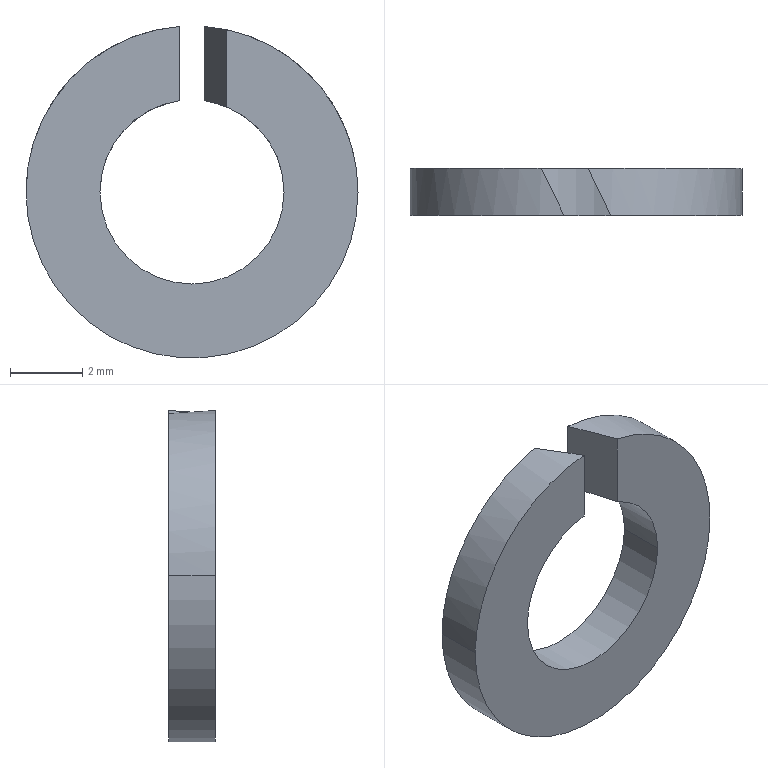Part | STEP file | ZZ24-M5 | 1 solid | 10 faces | box 9.2 x 1.3 x 9.188 mm | volume 56.371 mm3 | cylinder 6 | plane 4 | commonest cylinder face diameters 5.1 x3 9.2 x3
STEP:
#1=CARTESIAN_POINT('',(0.,0.,0.));
#2=DIRECTION('',(0.,0.,1.));
#3=DIRECTION('',(1.,0.,0.));
#4=AXIS2_PLACEMENT_3D('',#1,#2,#3);
#5=CARTESIAN_POINT('',(0.967,0.,2.36));
#6=VERTEX_POINT('',#5);
#7=CARTESIAN_POINT('',(0.333,1.3,2.528));
#8=VERTEX_POINT('',#7);
#9=CARTESIAN_POINT('',(0.967,0.,2.36));
#10=CARTESIAN_POINT('',(0.7635,0.4172,2.443));
#11=CARTESIAN_POINT('',(0.551,0.853,2.499));
#12=CARTESIAN_POINT('',(0.333,1.3,2.528));
#13=(BOUNDED_CURVE()B_SPLINE_CURVE(3,(#9,#10,#11,#12),.UNSPECIFIED.,.F.,.F.)B_SPLINE_CURVE_WITH_KNOTS((4,4),(1.182,1.44),.PIECEWISE_BEZIER_KNOTS.)CURVE()GEOMETRIC_REPRESENTATION_ITEM()RATIONAL_B_SPLINE_CURVE((1.,0.9945,0.9945,1.))REPRESENTATION_ITEM(''));
#14=CARTESIAN_POINT('',(0.,1.3,0.));
#15=DIRECTION('',(0.,-1.,0.));
#16=DIRECTION('',(-1.,0.,0.001512));
#17=AXIS2_PLACEMENT_3D('',#14,#15,#16);
#18=CYLINDRICAL_SURFACE('',#17,2.55);
#19=CARTESIAN_POINT('',(4.325,1.3));
#20=CARTESIAN_POINT('',(4.329,1.281));
#21=CARTESIAN_POINT('',(4.337,1.243));
#22=CARTESIAN_POINT('',(4.348,1.186));
#23=CARTESIAN_POINT('',(4.36,1.129));
#24=CARTESIAN_POINT('',(4.372,1.071));
#25=CARTESIAN_POINT('',(4.384,1.013));
#26=CARTESIAN_POINT('',(4.395,0.9553));
#27=CARTESIAN_POINT('',(4.407,0.8969));
#28=CARTESIAN_POINT('',(4.419,0.8383));
#29=CARTESIAN_POINT('',(4.43,0.7795));
#30=CARTESIAN_POINT('',(4.442,0.7204));
#31=CARTESIAN_POINT('',(4.454,0.6612));
#32=CARTESIAN_POINT('',(4.466,0.6018));
#33=CARTESIAN_POINT('',(4.477,0.5422));
#34=CARTESIAN_POINT('',(4.489,0.4824));
#35=CARTESIAN_POINT('',(4.501,0.4225));
#36=CARTESIAN_POINT('',(4.513,0.3624));
#37=CARTESIAN_POINT('',(4.524,0.3023));
#38=CARTESIAN_POINT('',(4.536,0.242));
#39=CARTESIAN_POINT('',(4.548,0.1816));
#40=CARTESIAN_POINT('',(4.56,0.1211));
#41=CARTESIAN_POINT('',(4.571,0.06061));
#42=CARTESIAN_POINT('',(4.579,0.02021));
#43=CARTESIAN_POINT('',(4.583,0.));
#44=B_SPLINE_CURVE_WITH_KNOTS('',3,(#19,#20,#21,#22,#23,#24,#25,#26,#27,#28,#29,#30,#31,#32,#33,#34,#35,#36,#37,#38,#39,#40,#41,#42,#43),.UNSPECIFIED.,.F.,.F.,(4,1,1,1,1,1,1,1,1,1,1,1,1,1,1,1,1,1,1,1,1,1,4),(1.182,1.194,1.205,1.217,1.229,1.24,1.252,1.264,1.276,1.287,1.299,1.311,1.323,1.334,1.346,1.358,1.369,1.381,1.393,1.405,1.416,1.428,1.44),.QUASI_UNIFORM_KNOTS.);
#45=(GEOMETRIC_REPRESENTATION_CONTEXT(2)PARAMETRIC_REPRESENTATION_CONTEXT()REPRESENTATION_CONTEXT('',''));
#46=DEFINITIONAL_REPRESENTATION('',(#44),#45);
#47=PCURVE('',#18,#46);
#48=CARTESIAN_POINT('',(0.967,0.,4.6));
#49=DIRECTION('',(-0.8988,-0.4384,0.));
#50=DIRECTION('',(0.4384,-0.8988,0.));
#51=AXIS2_PLACEMENT_3D('',#48,#49,#50);
#52=PLANE('',#51);
#53=CARTESIAN_POINT('',(0.,-2.24));
#54=CARTESIAN_POINT('',(-0.4642,-2.157));
#55=CARTESIAN_POINT('',(-0.949,-2.101));
#56=CARTESIAN_POINT('',(-1.446,-2.072));
#57=(BOUNDED_CURVE()B_SPLINE_CURVE(3,(#53,#54,#55,#56),.UNSPECIFIED.,.F.,.F.)B_SPLINE_CURVE_WITH_KNOTS((4,4),(1.182,1.44),.PIECEWISE_BEZIER_KNOTS.)CURVE()GEOMETRIC_REPRESENTATION_ITEM()RATIONAL_B_SPLINE_CURVE((1.,0.9945,0.9945,1.))REPRESENTATION_ITEM(''));
#58=(GEOMETRIC_REPRESENTATION_CONTEXT(2)PARAMETRIC_REPRESENTATION_CONTEXT()REPRESENTATION_CONTEXT('',''));
#59=DEFINITIONAL_REPRESENTATION('',(#57),#58);
#60=PCURVE('',#52,#59);
#61=SURFACE_CURVE('',#13,(#47,#60),.PCURVE_S1.);
#62=EDGE_CURVE('',#6,#8,#61,.T.);
#63=ORIENTED_EDGE('',*,*,#62,.F.);
#64=CARTESIAN_POINT('',(2.55,0.,-0.003856));
#65=VERTEX_POINT('',#64);
#66=CARTESIAN_POINT('',(0.,0.,0.));
#67=DIRECTION('',(0.,1.,0.));
#68=DIRECTION('',(1.,0.,-0.001512));
#69=AXIS2_PLACEMENT_3D('',#66,#67,#68);
#70=CIRCLE('',#69,2.55);
#71=CARTESIAN_POINT('',(9.425,1.3));
#72=DIRECTION('',(-1.,0.));
#73=VECTOR('',#72,1.);
#74=LINE('',#71,#73);
#75=(GEOMETRIC_REPRESENTATION_CONTEXT(2)PARAMETRIC_REPRESENTATION_CONTEXT()REPRESENTATION_CONTEXT('',''));
#76=DEFINITIONAL_REPRESENTATION('',(#74),#75);
#77=PCURVE('',#18,#76);
#78=CARTESIAN_POINT('',(0.,0.,0.));
#79=DIRECTION('',(0.,-1.,0.));
#80=DIRECTION('',(-1.,0.,0.001512));
#81=AXIS2_PLACEMENT_3D('',#78,#79,#80);
#82=PLANE('',#81);
#83=CARTESIAN_POINT('',(-2.55,0.));
#84=CARTESIAN_POINT('',(-2.55,4.417));
#85=CARTESIAN_POINT('',(1.275,2.208));
#86=CARTESIAN_POINT('',(5.1,0.));
#87=CARTESIAN_POINT('',(1.275,-2.208));
#88=CARTESIAN_POINT('',(-2.55,-4.417));
#89=CARTESIAN_POINT('',(-2.55,0.));
#90=(BOUNDED_CURVE()B_SPLINE_CURVE(2,(#83,#84,#85,#86,#87,#88,#89),.UNSPECIFIED.,.T.,.F.)B_SPLINE_CURVE_WITH_KNOTS((1,2,2,2,2,1),(-2.094,0.,2.094,4.189,6.283,8.378),.UNSPECIFIED.)CURVE()GEOMETRIC_REPRESENTATION_ITEM()RATIONAL_B_SPLINE_CURVE((1.,0.5,1.,0.5,1.,0.5,1.))REPRESENTATION_ITEM(''));
#91=(GEOMETRIC_REPRESENTATION_CONTEXT(2)PARAMETRIC_REPRESENTATION_CONTEXT()REPRESENTATION_CONTEXT('',''));
#92=DEFINITIONAL_REPRESENTATION('',(#90),#91);
#93=PCURVE('',#82,#92);
#94=SURFACE_CURVE('',#70,(#77,#93),.PCURVE_S1.);
#95=EDGE_CURVE('',#6,#65,#94,.T.);
#96=ORIENTED_EDGE('',*,*,#95,.T.);
#97=CARTESIAN_POINT('',(2.55,1.3,-0.003856));
#98=VERTEX_POINT('',#97);
#99=CARTESIAN_POINT('',(2.55,1.3,-0.003856));
#100=DIRECTION('',(0.,-1.,0.));
#101=VECTOR('',#100,1.);
#102=LINE('',#99,#101);
#103=CARTESIAN_POINT('',(3.142,0.));
#104=DIRECTION('',(0.,1.));
#105=VECTOR('',#104,1.);
#106=LINE('',#103,#105);
#107=(GEOMETRIC_REPRESENTATION_CONTEXT(2)PARAMETRIC_REPRESENTATION_CONTEXT()REPRESENTATION_CONTEXT('',''));
#108=DEFINITIONAL_REPRESENTATION('',(#106),#107);
#109=PCURVE('',#18,#108);
#110=CARTESIAN_POINT('',(0.,1.3,0.));
#111=DIRECTION('',(0.,-1.,0.));
#112=DIRECTION('',(-1.,0.,0.001512));
#113=AXIS2_PLACEMENT_3D('',#110,#111,#112);
#114=CYLINDRICAL_SURFACE('',#113,2.55);
#115=CARTESIAN_POINT('',(3.142,0.));
#116=DIRECTION('',(0.,1.));
#117=VECTOR('',#116,1.);
#118=LINE('',#115,#117);
#119=(GEOMETRIC_REPRESENTATION_CONTEXT(2)PARAMETRIC_REPRESENTATION_CONTEXT()REPRESENTATION_CONTEXT('',''));
#120=DEFINITIONAL_REPRESENTATION('',(#118),#119);
#121=PCURVE('',#114,#120);
#122=SURFACE_CURVE('',#102,(#109,#121),.PCURVE_S1.);
#123=EDGE_CURVE('',#98,#65,#122,.T.);
#124=ORIENTED_EDGE('',*,*,#123,.F.);
#125=CARTESIAN_POINT('',(0.,1.3,0.));
#126=DIRECTION('',(0.,-1.,0.));
#127=DIRECTION('',(-1.,0.,0.001512));
#128=AXIS2_PLACEMENT_3D('',#125,#126,#127);
#129=CIRCLE('',#128,2.55);
#130=CARTESIAN_POINT('',(0.,0.));
#131=DIRECTION('',(1.,0.));
#132=VECTOR('',#131,1.);
#133=LINE('',#130,#132);
#134=(GEOMETRIC_REPRESENTATION_CONTEXT(2)PARAMETRIC_REPRESENTATION_CONTEXT()REPRESENTATION_CONTEXT('',''));
#135=DEFINITIONAL_REPRESENTATION('',(#133),#134);
#136=PCURVE('',#18,#135);
#137=CARTESIAN_POINT('',(0.,1.3,0.));
#138=DIRECTION('',(0.,1.,0.));
#139=DIRECTION('',(1.,0.,-0.001512));
#140=AXIS2_PLACEMENT_3D('',#137,#138,#139);
#141=PLANE('',#140);
#142=CARTESIAN_POINT('',(-2.55,0.));
#143=CARTESIAN_POINT('',(-2.55,4.417));
#144=CARTESIAN_POINT('',(1.275,2.208));
#145=CARTESIAN_POINT('',(5.1,0.));
#146=CARTESIAN_POINT('',(1.275,-2.208));
#147=CARTESIAN_POINT('',(-2.55,-4.417));
#148=CARTESIAN_POINT('',(-2.55,0.));
#149=(BOUNDED_CURVE()B_SPLINE_CURVE(2,(#142,#143,#144,#145,#146,#147,#148),.UNSPECIFIED.,.T.,.F.)B_SPLINE_CURVE_WITH_KNOTS((1,2,2,2,2,1),(-2.094,0.,2.094,4.189,6.283,8.378),.UNSPECIFIED.)CURVE()GEOMETRIC_REPRESENTATION_ITEM()RATIONAL_B_SPLINE_CURVE((1.,0.5,1.,0.5,1.,0.5,1.))REPRESENTATION_ITEM(''));
#150=(GEOMETRIC_REPRESENTATION_CONTEXT(2)PARAMETRIC_REPRESENTATION_CONTEXT()REPRESENTATION_CONTEXT('',''));
#151=DEFINITIONAL_REPRESENTATION('',(#149),#150);
#152=PCURVE('',#141,#151);
#153=SURFACE_CURVE('',#129,(#136,#152),.PCURVE_S1.);
#154=EDGE_CURVE('',#98,#8,#153,.T.);
#155=ORIENTED_EDGE('',*,*,#154,.T.);
#156=EDGE_LOOP('',(#63,#96,#124,#155));
#157=FACE_BOUND('',#156,.F.);
#158=ADVANCED_FACE('',(#157),#18,.F.);
#159=CARTESIAN_POINT('',(-2.55,0.,0.003856));
#160=VERTEX_POINT('',#159);
#161=CARTESIAN_POINT('',(0.,0.,0.));
#162=DIRECTION('',(0.,1.,0.));
#163=DIRECTION('',(1.,0.,-0.001512));
#164=AXIS2_PLACEMENT_3D('',#161,#162,#163);
#165=CIRCLE('',#164,2.55);
#166=CARTESIAN_POINT('',(3.142,1.3));
#167=DIRECTION('',(-1.,0.));
#168=VECTOR('',#167,1.);
#169=LINE('',#166,#168);
#170=(GEOMETRIC_REPRESENTATION_CONTEXT(2)PARAMETRIC_REPRESENTATION_CONTEXT()REPRESENTATION_CONTEXT('',''));
#171=DEFINITIONAL_REPRESENTATION('',(#169),#170);
#172=PCURVE('',#114,#171);
#173=CARTESIAN_POINT('',(-2.55,0.));
#174=CARTESIAN_POINT('',(-2.55,4.417));
#175=CARTESIAN_POINT('',(1.275,2.208));
#176=CARTESIAN_POINT('',(5.1,0.));
#177=CARTESIAN_POINT('',(1.275,-2.208));
#178=CARTESIAN_POINT('',(-2.55,-4.417));
#179=CARTESIAN_POINT('',(-2.55,0.));
#180=(BOUNDED_CURVE()B_SPLINE_CURVE(2,(#173,#174,#175,#176,#177,#178,#179),.UNSPECIFIED.,.T.,.F.)B_SPLINE_CURVE_WITH_KNOTS((1,2,2,2,2,1),(-2.094,0.,2.094,4.189,6.283,8.378),.UNSPECIFIED.)CURVE()GEOMETRIC_REPRESENTATION_ITEM()RATIONAL_B_SPLINE_CURVE((1.,0.5,1.,0.5,1.,0.5,1.))REPRESENTATION_ITEM(''));
#181=(GEOMETRIC_REPRESENTATION_CONTEXT(2)PARAMETRIC_REPRESENTATION_CONTEXT()REPRESENTATION_CONTEXT('',''));
#182=DEFINITIONAL_REPRESENTATION('',(#180),#181);
#183=PCURVE('',#82,#182);
#184=SURFACE_CURVE('',#165,(#172,#183),.PCURVE_S1.);
#185=EDGE_CURVE('',#65,#160,#184,.T.);
#186=ORIENTED_EDGE('',*,*,#185,.T.);
#187=CARTESIAN_POINT('',(-2.55,1.3,0.003856));
#188=VERTEX_POINT('',#187);
#189=CARTESIAN_POINT('',(-2.55,1.3,0.003856));
#190=DIRECTION('',(0.,-1.,0.));
#191=VECTOR('',#190,1.);
#192=LINE('',#189,#191);
#193=CARTESIAN_POINT('',(0.,0.));
#194=DIRECTION('',(0.,1.));
#195=VECTOR('',#194,1.);
#196=LINE('',#193,#195);
#197=(GEOMETRIC_REPRESENTATION_CONTEXT(2)PARAMETRIC_REPRESENTATION_CONTEXT()REPRESENTATION_CONTEXT('',''));
#198=DEFINITIONAL_REPRESENTATION('',(#196),#197);
#199=PCURVE('',#114,#198);
#200=CARTESIAN_POINT('',(0.,1.3,0.));
#201=DIRECTION('',(0.,-1.,0.));
#202=DIRECTION('',(-1.,0.,0.001512));
#203=AXIS2_PLACEMENT_3D('',#200,#201,#202);
#204=CYLINDRICAL_SURFACE('',#203,2.55);
#205=CARTESIAN_POINT('',(6.283,0.));
#206=DIRECTION('',(0.,1.));
#207=VECTOR('',#206,1.);
#208=LINE('',#205,#207);
#209=(GEOMETRIC_REPRESENTATION_CONTEXT(2)PARAMETRIC_REPRESENTATION_CONTEXT()REPRESENTATION_CONTEXT('',''));
#210=DEFINITIONAL_REPRESENTATION('',(#208),#209);
#211=PCURVE('',#204,#210);
#212=SURFACE_CURVE('',#192,(#199,#211),.PCURVE_S1.);
#213=EDGE_CURVE('',#188,#160,#212,.T.);
#214=ORIENTED_EDGE('',*,*,#213,.F.);
#215=CARTESIAN_POINT('',(0.,1.3,0.));
#216=DIRECTION('',(0.,-1.,0.));
#217=DIRECTION('',(-1.,0.,0.001512));
#218=AXIS2_PLACEMENT_3D('',#215,#216,#217);
#219=CIRCLE('',#218,2.55);
#220=CARTESIAN_POINT('',(0.,0.));
#221=DIRECTION('',(1.,0.));
#222=VECTOR('',#221,1.);
#223=LINE('',#220,#222);
#224=(GEOMETRIC_REPRESENTATION_CONTEXT(2)PARAMETRIC_REPRESENTATION_CONTEXT()REPRESENTATION_CONTEXT('',''));
#225=DEFINITIONAL_REPRESENTATION('',(#223),#224);
#226=PCURVE('',#114,#225);
#227=CARTESIAN_POINT('',(-2.55,0.));
#228=CARTESIAN_POINT('',(-2.55,4.417));
#229=CARTESIAN_POINT('',(1.275,2.208));
#230=CARTESIAN_POINT('',(5.1,0.));
#231=CARTESIAN_POINT('',(1.275,-2.208));
#232=CARTESIAN_POINT('',(-2.55,-4.417));
#233=CARTESIAN_POINT('',(-2.55,0.));
#234=(BOUNDED_CURVE()B_SPLINE_CURVE(2,(#227,#228,#229,#230,#231,#232,#233),.UNSPECIFIED.,.T.,.F.)B_SPLINE_CURVE_WITH_KNOTS((1,2,2,2,2,1),(-2.094,0.,2.094,4.189,6.283,8.378),.UNSPECIFIED.)CURVE()GEOMETRIC_REPRESENTATION_ITEM()RATIONAL_B_SPLINE_CURVE((1.,0.5,1.,0.5,1.,0.5,1.))REPRESENTATION_ITEM(''));
#235=(GEOMETRIC_REPRESENTATION_CONTEXT(2)PARAMETRIC_REPRESENTATION_CONTEXT()REPRESENTATION_CONTEXT('',''));
#236=DEFINITIONAL_REPRESENTATION('',(#234),#235);
#237=PCURVE('',#141,#236);
#238=SURFACE_CURVE('',#219,(#226,#237),.PCURVE_S1.);
#239=EDGE_CURVE('',#188,#98,#238,.T.);
#240=ORIENTED_EDGE('',*,*,#239,.T.);
#241=ORIENTED_EDGE('',*,*,#123,.T.);
#242=EDGE_LOOP('',(#186,#214,#240,#241));
#243=FACE_BOUND('',#242,.F.);
#244=ADVANCED_FACE('',(#243),#114,.F.);
#245=CARTESIAN_POINT('',(-4.6,1.3,0.006956));
#246=VERTEX_POINT('',#245);
#247=CARTESIAN_POINT('',(4.6,1.3,-0.006956));
#248=VERTEX_POINT('',#247);
#249=CARTESIAN_POINT('',(0.,1.3,0.));
#250=DIRECTION('',(0.,-1.,0.));
#251=DIRECTION('',(-1.,0.,0.001512));
#252=AXIS2_PLACEMENT_3D('',#249,#250,#251);
#253=CIRCLE('',#252,4.6);
#254=CARTESIAN_POINT('',(0.,1.3,0.));
#255=DIRECTION('',(0.,-1.,0.));
#256=DIRECTION('',(-1.,0.,0.001512));
#257=AXIS2_PLACEMENT_3D('',#254,#255,#256);
#258=CYLINDRICAL_SURFACE('',#257,4.6);
#259=CARTESIAN_POINT('',(0.,0.));
#260=DIRECTION('',(1.,0.));
#261=VECTOR('',#260,1.);
#262=LINE('',#259,#261);
#263=(GEOMETRIC_REPRESENTATION_CONTEXT(2)PARAMETRIC_REPRESENTATION_CONTEXT()REPRESENTATION_CONTEXT('',''));
#264=DEFINITIONAL_REPRESENTATION('',(#262),#263);
#265=PCURVE('',#258,#264);
#266=CARTESIAN_POINT('',(-4.6,0.));
#267=CARTESIAN_POINT('',(-4.6,7.967));
#268=CARTESIAN_POINT('',(2.3,3.984));
#269=CARTESIAN_POINT('',(9.2,0.));
#270=CARTESIAN_POINT('',(2.3,-3.984));
#271=CARTESIAN_POINT('',(-4.6,-7.967));
#272=CARTESIAN_POINT('',(-4.6,0.));
#273=(BOUNDED_CURVE()B_SPLINE_CURVE(2,(#266,#267,#268,#269,#270,#271,#272),.UNSPECIFIED.,.T.,.F.)B_SPLINE_CURVE_WITH_KNOTS((1,2,2,2,2,1),(-2.094,0.,2.094,4.189,6.283,8.378),.UNSPECIFIED.)CURVE()GEOMETRIC_REPRESENTATION_ITEM()RATIONAL_B_SPLINE_CURVE((1.,0.5,1.,0.5,1.,0.5,1.))REPRESENTATION_ITEM(''));
#274=(GEOMETRIC_REPRESENTATION_CONTEXT(2)PARAMETRIC_REPRESENTATION_CONTEXT()REPRESENTATION_CONTEXT('',''));
#275=DEFINITIONAL_REPRESENTATION('',(#273),#274);
#276=PCURVE('',#141,#275);
#277=SURFACE_CURVE('',#253,(#265,#276),.PCURVE_S1.);
#278=EDGE_CURVE('',#246,#248,#277,.T.);
#279=ORIENTED_EDGE('',*,*,#278,.T.);
#280=CARTESIAN_POINT('',(4.6,0.,-0.006956));
#281=VERTEX_POINT('',#280);
#282=CARTESIAN_POINT('',(4.6,1.3,-0.006956));
#283=DIRECTION('',(0.,-1.,0.));
#284=VECTOR('',#283,1.);
#285=LINE('',#282,#284);
#286=CARTESIAN_POINT('',(3.142,0.));
#287=DIRECTION('',(0.,1.));
#288=VECTOR('',#287,1.);
#289=LINE('',#286,#288);
#290=(GEOMETRIC_REPRESENTATION_CONTEXT(2)PARAMETRIC_REPRESENTATION_CONTEXT()REPRESENTATION_CONTEXT('',''));
#291=DEFINITIONAL_REPRESENTATION('',(#289),#290);
#292=PCURVE('',#258,#291);
#293=CARTESIAN_POINT('',(0.,1.3,0.));
#294=DIRECTION('',(0.,-1.,0.));
#295=DIRECTION('',(-1.,0.,0.001512));
#296=AXIS2_PLACEMENT_3D('',#293,#294,#295);
#297=CYLINDRICAL_SURFACE('',#296,4.6);
#298=CARTESIAN_POINT('',(3.142,0.));
#299=DIRECTION('',(0.,1.));
#300=VECTOR('',#299,1.);
#301=LINE('',#298,#300);
#302=(GEOMETRIC_REPRESENTATION_CONTEXT(2)PARAMETRIC_REPRESENTATION_CONTEXT()REPRESENTATION_CONTEXT('',''));
#303=DEFINITIONAL_REPRESENTATION('',(#301),#302);
#304=PCURVE('',#297,#303);
#305=SURFACE_CURVE('',#285,(#292,#304),.PCURVE_S1.);
#306=EDGE_CURVE('',#248,#281,#305,.T.);
#307=ORIENTED_EDGE('',*,*,#306,.T.);
#308=CARTESIAN_POINT('',(-4.6,0.,0.006956));
#309=VERTEX_POINT('',#308);
#310=CARTESIAN_POINT('',(0.,0.,0.));
#311=DIRECTION('',(0.,1.,0.));
#312=DIRECTION('',(1.,0.,-0.001512));
#313=AXIS2_PLACEMENT_3D('',#310,#311,#312);
#314=CIRCLE('',#313,4.6);
#315=CARTESIAN_POINT('',(3.142,1.3));
#316=DIRECTION('',(-1.,0.));
#317=VECTOR('',#316,1.);
#318=LINE('',#315,#317);
#319=(GEOMETRIC_REPRESENTATION_CONTEXT(2)PARAMETRIC_REPRESENTATION_CONTEXT()REPRESENTATION_CONTEXT('',''));
#320=DEFINITIONAL_REPRESENTATION('',(#318),#319);
#321=PCURVE('',#258,#320);
#322=CARTESIAN_POINT('',(-4.6,0.));
#323=CARTESIAN_POINT('',(-4.6,7.967));
#324=CARTESIAN_POINT('',(2.3,3.984));
#325=CARTESIAN_POINT('',(9.2,0.));
#326=CARTESIAN_POINT('',(2.3,-3.984));
#327=CARTESIAN_POINT('',(-4.6,-7.967));
#328=CARTESIAN_POINT('',(-4.6,0.));
#329=(BOUNDED_CURVE()B_SPLINE_CURVE(2,(#322,#323,#324,#325,#326,#327,#328),.UNSPECIFIED.,.T.,.F.)B_SPLINE_CURVE_WITH_KNOTS((1,2,2,2,2,1),(-2.094,0.,2.094,4.189,6.283,8.378),.UNSPECIFIED.)CURVE()GEOMETRIC_REPRESENTATION_ITEM()RATIONAL_B_SPLINE_CURVE((1.,0.5,1.,0.5,1.,0.5,1.))REPRESENTATION_ITEM(''));
#330=(GEOMETRIC_REPRESENTATION_CONTEXT(2)PARAMETRIC_REPRESENTATION_CONTEXT()REPRESENTATION_CONTEXT('',''));
#331=DEFINITIONAL_REPRESENTATION('',(#329),#330);
#332=PCURVE('',#82,#331);
#333=SURFACE_CURVE('',#314,(#321,#332),.PCURVE_S1.);
#334=EDGE_CURVE('',#281,#309,#333,.T.);
#335=ORIENTED_EDGE('',*,*,#334,.T.);
#336=CARTESIAN_POINT('',(-4.6,1.3,0.006956));
#337=DIRECTION('',(0.,-1.,0.));
#338=VECTOR('',#337,1.);
#339=LINE('',#336,#338);
#340=CARTESIAN_POINT('',(0.,0.));
#341=DIRECTION('',(0.,1.));
#342=VECTOR('',#341,1.);
#343=LINE('',#340,#342);
#344=(GEOMETRIC_REPRESENTATION_CONTEXT(2)PARAMETRIC_REPRESENTATION_CONTEXT()REPRESENTATION_CONTEXT('',''));
#345=DEFINITIONAL_REPRESENTATION('',(#343),#344);
#346=PCURVE('',#258,#345);
#347=CARTESIAN_POINT('',(0.,1.3,0.));
#348=DIRECTION('',(0.,-1.,0.));
#349=DIRECTION('',(-1.,0.,0.001512));
#350=AXIS2_PLACEMENT_3D('',#347,#348,#349);
#351=CYLINDRICAL_SURFACE('',#350,4.6);
#352=CARTESIAN_POINT('',(6.283,0.));
#353=DIRECTION('',(0.,1.));
#354=VECTOR('',#353,1.);
#355=LINE('',#352,#354);
#356=(GEOMETRIC_REPRESENTATION_CONTEXT(2)PARAMETRIC_REPRESENTATION_CONTEXT()REPRESENTATION_CONTEXT('',''));
#357=DEFINITIONAL_REPRESENTATION('',(#355),#356);
#358=PCURVE('',#351,#357);
#359=SURFACE_CURVE('',#339,(#346,#358),.PCURVE_S1.);
#360=EDGE_CURVE('',#246,#309,#359,.T.);
#361=ORIENTED_EDGE('',*,*,#360,.F.);
#362=EDGE_LOOP('',(#279,#307,#335,#361));
#363=FACE_BOUND('',#362,.T.);
#364=ADVANCED_FACE('',(#363),#258,.T.);
#365=CARTESIAN_POINT('',(-0.967,1.3,4.497));
#366=VERTEX_POINT('',#365);
#367=CARTESIAN_POINT('',(0.,1.3,0.));
#368=DIRECTION('',(0.,-1.,0.));
#369=DIRECTION('',(-1.,0.,0.001512));
#370=AXIS2_PLACEMENT_3D('',#367,#368,#369);
#371=CIRCLE('',#370,4.6);
#372=CARTESIAN_POINT('',(0.,0.));
#373=DIRECTION('',(1.,0.));
#374=VECTOR('',#373,1.);
#375=LINE('',#372,#374);
#376=(GEOMETRIC_REPRESENTATION_CONTEXT(2)PARAMETRIC_REPRESENTATION_CONTEXT()REPRESENTATION_CONTEXT('',''));
#377=DEFINITIONAL_REPRESENTATION('',(#375),#376);
#378=PCURVE('',#351,#377);
#379=CARTESIAN_POINT('',(-4.6,0.));
#380=CARTESIAN_POINT('',(-4.6,7.967));
#381=CARTESIAN_POINT('',(2.3,3.984));
#382=CARTESIAN_POINT('',(9.2,0.));
#383=CARTESIAN_POINT('',(2.3,-3.984));
#384=CARTESIAN_POINT('',(-4.6,-7.967));
#385=CARTESIAN_POINT('',(-4.6,0.));
#386=(BOUNDED_CURVE()B_SPLINE_CURVE(2,(#379,#380,#381,#382,#383,#384,#385),.UNSPECIFIED.,.T.,.F.)B_SPLINE_CURVE_WITH_KNOTS((1,2,2,2,2,1),(-2.094,0.,2.094,4.189,6.283,8.378),.UNSPECIFIED.)CURVE()GEOMETRIC_REPRESENTATION_ITEM()RATIONAL_B_SPLINE_CURVE((1.,0.5,1.,0.5,1.,0.5,1.))REPRESENTATION_ITEM(''));
#387=(GEOMETRIC_REPRESENTATION_CONTEXT(2)PARAMETRIC_REPRESENTATION_CONTEXT()REPRESENTATION_CONTEXT('',''));
#388=DEFINITIONAL_REPRESENTATION('',(#386),#387);
#389=PCURVE('',#141,#388);
#390=SURFACE_CURVE('',#371,(#378,#389),.PCURVE_S1.);
#391=EDGE_CURVE('',#366,#246,#390,.T.);
#392=ORIENTED_EDGE('',*,*,#391,.T.);
#393=ORIENTED_EDGE('',*,*,#360,.T.);
#394=CARTESIAN_POINT('',(-0.333,0.,4.588));
#395=VERTEX_POINT('',#394);
#396=CARTESIAN_POINT('',(0.,0.,0.));
#397=DIRECTION('',(0.,1.,0.));
#398=DIRECTION('',(1.,0.,-0.001512));
#399=AXIS2_PLACEMENT_3D('',#396,#397,#398);
#400=CIRCLE('',#399,4.6);
#401=CARTESIAN_POINT('',(9.425,1.3));
#402=DIRECTION('',(-1.,0.));
#403=VECTOR('',#402,1.);
#404=LINE('',#401,#403);
#405=(GEOMETRIC_REPRESENTATION_CONTEXT(2)PARAMETRIC_REPRESENTATION_CONTEXT()REPRESENTATION_CONTEXT('',''));
#406=DEFINITIONAL_REPRESENTATION('',(#404),#405);
#407=PCURVE('',#351,#406);
#408=CARTESIAN_POINT('',(-4.6,0.));
#409=CARTESIAN_POINT('',(-4.6,7.967));
#410=CARTESIAN_POINT('',(2.3,3.984));
#411=CARTESIAN_POINT('',(9.2,0.));
#412=CARTESIAN_POINT('',(2.3,-3.984));
#413=CARTESIAN_POINT('',(-4.6,-7.967));
#414=CARTESIAN_POINT('',(-4.6,0.));
#415=(BOUNDED_CURVE()B_SPLINE_CURVE(2,(#408,#409,#410,#411,#412,#413,#414),.UNSPECIFIED.,.T.,.F.)B_SPLINE_CURVE_WITH_KNOTS((1,2,2,2,2,1),(-2.094,0.,2.094,4.189,6.283,8.378),.UNSPECIFIED.)CURVE()GEOMETRIC_REPRESENTATION_ITEM()RATIONAL_B_SPLINE_CURVE((1.,0.5,1.,0.5,1.,0.5,1.))REPRESENTATION_ITEM(''));
#416=(GEOMETRIC_REPRESENTATION_CONTEXT(2)PARAMETRIC_REPRESENTATION_CONTEXT()REPRESENTATION_CONTEXT('',''));
#417=DEFINITIONAL_REPRESENTATION('',(#415),#416);
#418=PCURVE('',#82,#417);
#419=SURFACE_CURVE('',#400,(#407,#418),.PCURVE_S1.);
#420=EDGE_CURVE('',#309,#395,#419,.T.);
#421=ORIENTED_EDGE('',*,*,#420,.T.);
#422=CARTESIAN_POINT('',(-0.333,0.,4.588));
#423=CARTESIAN_POINT('',(-0.5463,0.4373,4.572));
#424=CARTESIAN_POINT('',(-0.758,0.8713,4.542));
#425=CARTESIAN_POINT('',(-0.967,1.3,4.497));
#426=(BOUNDED_CURVE()B_SPLINE_CURVE(3,(#422,#423,#424,#425),.UNSPECIFIED.,.F.,.F.)B_SPLINE_CURVE_WITH_KNOTS((4,4),(1.643,1.783),.PIECEWISE_BEZIER_KNOTS.)CURVE()GEOMETRIC_REPRESENTATION_ITEM()RATIONAL_B_SPLINE_CURVE((1.,0.9984,0.9984,1.))REPRESENTATION_ITEM(''));
#427=CARTESIAN_POINT('',(4.786,1.3));
#428=CARTESIAN_POINT('',(4.788,1.28));
#429=CARTESIAN_POINT('',(4.793,1.24));
#430=CARTESIAN_POINT('',(4.799,1.181));
#431=CARTESIAN_POINT('',(4.805,1.121));
#432=CARTESIAN_POINT('',(4.812,1.062));
#433=CARTESIAN_POINT('',(4.818,1.003));
#434=CARTESIAN_POINT('',(4.824,0.9432));
#435=CARTESIAN_POINT('',(4.831,0.8838));
#436=CARTESIAN_POINT('',(4.837,0.8245));
#437=CARTESIAN_POINT('',(4.843,0.7652));
#438=CARTESIAN_POINT('',(4.85,0.7059));
#439=CARTESIAN_POINT('',(4.856,0.6467));
#440=CARTESIAN_POINT('',(4.862,0.5876));
#441=CARTESIAN_POINT('',(4.869,0.5285));
#442=CARTESIAN_POINT('',(4.875,0.4695));
#443=CARTESIAN_POINT('',(4.881,0.4106));
#444=CARTESIAN_POINT('',(4.888,0.3517));
#445=CARTESIAN_POINT('',(4.894,0.2929));
#446=CARTESIAN_POINT('',(4.9,0.2341));
#447=CARTESIAN_POINT('',(4.907,0.1755));
#448=CARTESIAN_POINT('',(4.913,0.1169));
#449=CARTESIAN_POINT('',(4.919,0.05839));
#450=CARTESIAN_POINT('',(4.924,0.01945));
#451=CARTESIAN_POINT('',(4.926,0.));
#452=B_SPLINE_CURVE_WITH_KNOTS('',3,(#427,#428,#429,#430,#431,#432,#433,#434,#435,#436,#437,#438,#439,#440,#441,#442,#443,#444,#445,#446,#447,#448,#449,#450,#451),.UNSPECIFIED.,.F.,.F.,(4,1,1,1,1,1,1,1,1,1,1,1,1,1,1,1,1,1,1,1,1,1,4),(1.643,1.65,1.656,1.662,1.669,1.675,1.681,1.688,1.694,1.7,1.707,1.713,1.719,1.726,1.732,1.738,1.745,1.751,1.757,1.764,1.77,1.776,1.783),.QUASI_UNIFORM_KNOTS.);
#453=(GEOMETRIC_REPRESENTATION_CONTEXT(2)PARAMETRIC_REPRESENTATION_CONTEXT()REPRESENTATION_CONTEXT('',''));
#454=DEFINITIONAL_REPRESENTATION('',(#452),#453);
#455=PCURVE('',#351,#454);
#456=CARTESIAN_POINT('',(-0.967,1.3,4.6));
#457=DIRECTION('',(0.8988,0.4384,0.));
#458=DIRECTION('',(-0.4384,0.8988,0.));
#459=AXIS2_PLACEMENT_3D('',#456,#457,#458);
#460=PLANE('',#459);
#461=CARTESIAN_POINT('',(-1.446,-0.01207));
#462=CARTESIAN_POINT('',(-0.9598,-0.02755));
#463=CARTESIAN_POINT('',(-0.4769,-0.05784));
#464=CARTESIAN_POINT('',(0.,-0.1028));
#465=(BOUNDED_CURVE()B_SPLINE_CURVE(3,(#461,#462,#463,#464),.UNSPECIFIED.,.F.,.F.)B_SPLINE_CURVE_WITH_KNOTS((4,4),(1.643,1.783),.PIECEWISE_BEZIER_KNOTS.)CURVE()GEOMETRIC_REPRESENTATION_ITEM()RATIONAL_B_SPLINE_CURVE((1.,0.9984,0.9984,1.))REPRESENTATION_ITEM(''));
#466=(GEOMETRIC_REPRESENTATION_CONTEXT(2)PARAMETRIC_REPRESENTATION_CONTEXT()REPRESENTATION_CONTEXT('',''));
#467=DEFINITIONAL_REPRESENTATION('',(#465),#466);
#468=PCURVE('',#460,#467);
#469=SURFACE_CURVE('',#426,(#455,#468),.PCURVE_S1.);
#470=EDGE_CURVE('',#395,#366,#469,.T.);
#471=ORIENTED_EDGE('',*,*,#470,.T.);
#472=EDGE_LOOP('',(#392,#393,#421,#471));
#473=FACE_BOUND('',#472,.T.);
#474=ADVANCED_FACE('',(#473),#351,.T.);
#475=CARTESIAN_POINT('',(-0.333,0.,2.528));
#476=VERTEX_POINT('',#475);
#477=CARTESIAN_POINT('',(-0.333,0.,4.6));
#478=DIRECTION('',(0.,0.,-1.));
#479=VECTOR('',#478,1.);
#480=LINE('',#477,#479);
#481=CARTESIAN_POINT('',(0.3399,-4.599));
#482=DIRECTION('',(-0.001512,1.));
#483=VECTOR('',#482,1.);
#484=LINE('',#481,#483);
#485=(GEOMETRIC_REPRESENTATION_CONTEXT(2)PARAMETRIC_REPRESENTATION_CONTEXT()REPRESENTATION_CONTEXT('',''));
#486=DEFINITIONAL_REPRESENTATION('',(#484),#485);
#487=PCURVE('',#82,#486);
#488=CARTESIAN_POINT('',(-1.446,0.));
#489=DIRECTION('',(0.,-1.));
#490=VECTOR('',#489,1.);
#491=LINE('',#488,#490);
#492=(GEOMETRIC_REPRESENTATION_CONTEXT(2)PARAMETRIC_REPRESENTATION_CONTEXT()REPRESENTATION_CONTEXT('',''));
#493=DEFINITIONAL_REPRESENTATION('',(#491),#492);
#494=PCURVE('',#460,#493);
#495=SURFACE_CURVE('',#480,(#487,#494),.PCURVE_S1.);
#496=EDGE_CURVE('',#395,#476,#495,.T.);
#497=ORIENTED_EDGE('',*,*,#496,.F.);
#498=ORIENTED_EDGE('',*,*,#420,.F.);
#499=ORIENTED_EDGE('',*,*,#334,.F.);
#500=CARTESIAN_POINT('',(0.967,0.,4.497));
#501=VERTEX_POINT('',#500);
#502=CARTESIAN_POINT('',(0.,0.,0.));
#503=DIRECTION('',(0.,1.,0.));
#504=DIRECTION('',(1.,0.,-0.001512));
#505=AXIS2_PLACEMENT_3D('',#502,#503,#504);
#506=CIRCLE('',#505,4.6);
#507=CARTESIAN_POINT('',(-4.6,0.));
#508=CARTESIAN_POINT('',(-4.6,7.967));
#509=CARTESIAN_POINT('',(2.3,3.984));
#510=CARTESIAN_POINT('',(9.2,0.));
#511=CARTESIAN_POINT('',(2.3,-3.984));
#512=CARTESIAN_POINT('',(-4.6,-7.967));
#513=CARTESIAN_POINT('',(-4.6,0.));
#514=(BOUNDED_CURVE()B_SPLINE_CURVE(2,(#507,#508,#509,#510,#511,#512,#513),.UNSPECIFIED.,.T.,.F.)B_SPLINE_CURVE_WITH_KNOTS((1,2,2,2,2,1),(-2.094,0.,2.094,4.189,6.283,8.378),.UNSPECIFIED.)CURVE()GEOMETRIC_REPRESENTATION_ITEM()RATIONAL_B_SPLINE_CURVE((1.,0.5,1.,0.5,1.,0.5,1.))REPRESENTATION_ITEM(''));
#515=(GEOMETRIC_REPRESENTATION_CONTEXT(2)PARAMETRIC_REPRESENTATION_CONTEXT()REPRESENTATION_CONTEXT('',''));
#516=DEFINITIONAL_REPRESENTATION('',(#514),#515);
#517=PCURVE('',#82,#516);
#518=CARTESIAN_POINT('',(9.425,1.3));
#519=DIRECTION('',(-1.,0.));
#520=VECTOR('',#519,1.);
#521=LINE('',#518,#520);
#522=(GEOMETRIC_REPRESENTATION_CONTEXT(2)PARAMETRIC_REPRESENTATION_CONTEXT()REPRESENTATION_CONTEXT('',''));
#523=DEFINITIONAL_REPRESENTATION('',(#521),#522);
#524=PCURVE('',#297,#523);
#525=SURFACE_CURVE('',#506,(#517,#524),.PCURVE_S1.);
#526=EDGE_CURVE('',#501,#281,#525,.T.);
#527=ORIENTED_EDGE('',*,*,#526,.F.);
#528=CARTESIAN_POINT('',(0.967,0.,4.6));
#529=DIRECTION('',(0.,0.,-1.));
#530=VECTOR('',#529,1.);
#531=LINE('',#528,#530);
#532=CARTESIAN_POINT('',(-0.9601,-4.601));
#533=DIRECTION('',(-0.001512,1.));
#534=VECTOR('',#533,1.);
#535=LINE('',#532,#534);
#536=(GEOMETRIC_REPRESENTATION_CONTEXT(2)PARAMETRIC_REPRESENTATION_CONTEXT()REPRESENTATION_CONTEXT('',''));
#537=DEFINITIONAL_REPRESENTATION('',(#535),#536);
#538=PCURVE('',#82,#537);
#539=CARTESIAN_POINT('',(0.,0.));
#540=DIRECTION('',(0.,-1.));
#541=VECTOR('',#540,1.);
#542=LINE('',#539,#541);
#543=(GEOMETRIC_REPRESENTATION_CONTEXT(2)PARAMETRIC_REPRESENTATION_CONTEXT()REPRESENTATION_CONTEXT('',''));
#544=DEFINITIONAL_REPRESENTATION('',(#542),#543);
#545=PCURVE('',#52,#544);
#546=SURFACE_CURVE('',#531,(#538,#545),.PCURVE_S1.);
#547=EDGE_CURVE('',#501,#6,#546,.T.);
#548=ORIENTED_EDGE('',*,*,#547,.T.);
#549=ORIENTED_EDGE('',*,*,#95,.T.);
#550=ORIENTED_EDGE('',*,*,#185,.T.);
#551=CARTESIAN_POINT('',(0.,0.,0.));
#552=DIRECTION('',(0.,1.,0.));
#553=DIRECTION('',(1.,0.,-0.001512));
#554=AXIS2_PLACEMENT_3D('',#551,#552,#553);
#555=CIRCLE('',#554,2.55);
#556=CARTESIAN_POINT('',(-2.55,0.));
#557=CARTESIAN_POINT('',(-2.55,4.417));
#558=CARTESIAN_POINT('',(1.275,2.208));
#559=CARTESIAN_POINT('',(5.1,0.));
#560=CARTESIAN_POINT('',(1.275,-2.208));
#561=CARTESIAN_POINT('',(-2.55,-4.417));
#562=CARTESIAN_POINT('',(-2.55,0.));
#563=(BOUNDED_CURVE()B_SPLINE_CURVE(2,(#556,#557,#558,#559,#560,#561,#562),.UNSPECIFIED.,.T.,.F.)B_SPLINE_CURVE_WITH_KNOTS((1,2,2,2,2,1),(-2.094,0.,2.094,4.189,6.283,8.378),.UNSPECIFIED.)CURVE()GEOMETRIC_REPRESENTATION_ITEM()RATIONAL_B_SPLINE_CURVE((1.,0.5,1.,0.5,1.,0.5,1.))REPRESENTATION_ITEM(''));
#564=(GEOMETRIC_REPRESENTATION_CONTEXT(2)PARAMETRIC_REPRESENTATION_CONTEXT()REPRESENTATION_CONTEXT('',''));
#565=DEFINITIONAL_REPRESENTATION('',(#563),#564);
#566=PCURVE('',#82,#565);
#567=CARTESIAN_POINT('',(9.425,1.3));
#568=DIRECTION('',(-1.,0.));
#569=VECTOR('',#568,1.);
#570=LINE('',#567,#569);
#571=(GEOMETRIC_REPRESENTATION_CONTEXT(2)PARAMETRIC_REPRESENTATION_CONTEXT()REPRESENTATION_CONTEXT('',''));
#572=DEFINITIONAL_REPRESENTATION('',(#570),#571);
#573=PCURVE('',#204,#572);
#574=SURFACE_CURVE('',#555,(#566,#573),.PCURVE_S1.);
#575=EDGE_CURVE('',#160,#476,#574,.T.);
#576=ORIENTED_EDGE('',*,*,#575,.T.);
#577=EDGE_LOOP('',(#497,#498,#499,#527,#548,#549,#550,#576));
#578=FACE_BOUND('',#577,.T.);
#579=ADVANCED_FACE('',(#578),#82,.T.);
#580=CARTESIAN_POINT('',(0.333,1.3,4.588));
#581=VERTEX_POINT('',#580);
#582=CARTESIAN_POINT('',(0.333,1.3,4.6));
#583=DIRECTION('',(0.,0.,-1.));
#584=VECTOR('',#583,1.);
#585=LINE('',#582,#584);
#586=CARTESIAN_POINT('',(0.326,-4.6));
#587=DIRECTION('',(0.001512,1.));
#588=VECTOR('',#587,1.);
#589=LINE('',#586,#588);
#590=(GEOMETRIC_REPRESENTATION_CONTEXT(2)PARAMETRIC_REPRESENTATION_CONTEXT()REPRESENTATION_CONTEXT('',''));
#591=DEFINITIONAL_REPRESENTATION('',(#589),#590);
#592=PCURVE('',#141,#591);
#593=CARTESIAN_POINT('',(-1.446,0.));
#594=DIRECTION('',(0.,-1.));
#595=VECTOR('',#594,1.);
#596=LINE('',#593,#595);
#597=(GEOMETRIC_REPRESENTATION_CONTEXT(2)PARAMETRIC_REPRESENTATION_CONTEXT()REPRESENTATION_CONTEXT('',''));
#598=DEFINITIONAL_REPRESENTATION('',(#596),#597);
#599=PCURVE('',#52,#598);
#600=SURFACE_CURVE('',#585,(#592,#599),.PCURVE_S1.);
#601=EDGE_CURVE('',#581,#8,#600,.T.);
#602=ORIENTED_EDGE('',*,*,#601,.F.);
#603=CARTESIAN_POINT('',(0.,1.3,0.));
#604=DIRECTION('',(0.,-1.,0.));
#605=DIRECTION('',(-1.,0.,0.001512));
#606=AXIS2_PLACEMENT_3D('',#603,#604,#605);
#607=CIRCLE('',#606,4.6);
#608=CARTESIAN_POINT('',(-4.6,0.));
#609=CARTESIAN_POINT('',(-4.6,7.967));
#610=CARTESIAN_POINT('',(2.3,3.984));
#611=CARTESIAN_POINT('',(9.2,0.));
#612=CARTESIAN_POINT('',(2.3,-3.984));
#613=CARTESIAN_POINT('',(-4.6,-7.967));
#614=CARTESIAN_POINT('',(-4.6,0.));
#615=(BOUNDED_CURVE()B_SPLINE_CURVE(2,(#608,#609,#610,#611,#612,#613,#614),.UNSPECIFIED.,.T.,.F.)B_SPLINE_CURVE_WITH_KNOTS((1,2,2,2,2,1),(-2.094,0.,2.094,4.189,6.283,8.378),.UNSPECIFIED.)CURVE()GEOMETRIC_REPRESENTATION_ITEM()RATIONAL_B_SPLINE_CURVE((1.,0.5,1.,0.5,1.,0.5,1.))REPRESENTATION_ITEM(''));
#616=(GEOMETRIC_REPRESENTATION_CONTEXT(2)PARAMETRIC_REPRESENTATION_CONTEXT()REPRESENTATION_CONTEXT('',''));
#617=DEFINITIONAL_REPRESENTATION('',(#615),#616);
#618=PCURVE('',#141,#617);
#619=CARTESIAN_POINT('',(0.,0.));
#620=DIRECTION('',(1.,0.));
#621=VECTOR('',#620,1.);
#622=LINE('',#619,#621);
#623=(GEOMETRIC_REPRESENTATION_CONTEXT(2)PARAMETRIC_REPRESENTATION_CONTEXT()REPRESENTATION_CONTEXT('',''));
#624=DEFINITIONAL_REPRESENTATION('',(#622),#623);
#625=PCURVE('',#297,#624);
#626=SURFACE_CURVE('',#607,(#618,#625),.PCURVE_S1.);
#627=EDGE_CURVE('',#248,#581,#626,.T.);
#628=ORIENTED_EDGE('',*,*,#627,.F.);
#629=ORIENTED_EDGE('',*,*,#278,.F.);
#630=ORIENTED_EDGE('',*,*,#391,.F.);
#631=CARTESIAN_POINT('',(-0.967,1.3,2.36));
#632=VERTEX_POINT('',#631);
#633=CARTESIAN_POINT('',(-0.967,1.3,4.6));
#634=DIRECTION('',(0.,0.,-1.));
#635=VECTOR('',#634,1.);
#636=LINE('',#633,#635);
#637=CARTESIAN_POINT('',(-0.974,-4.599));
#638=DIRECTION('',(0.001512,1.));
#639=VECTOR('',#638,1.);
#640=LINE('',#637,#639);
#641=(GEOMETRIC_REPRESENTATION_CONTEXT(2)PARAMETRIC_REPRESENTATION_CONTEXT()REPRESENTATION_CONTEXT('',''));
#642=DEFINITIONAL_REPRESENTATION('',(#640),#641);
#643=PCURVE('',#141,#642);
#644=CARTESIAN_POINT('',(0.,0.));
#645=DIRECTION('',(0.,-1.));
#646=VECTOR('',#645,1.);
#647=LINE('',#644,#646);
#648=(GEOMETRIC_REPRESENTATION_CONTEXT(2)PARAMETRIC_REPRESENTATION_CONTEXT()REPRESENTATION_CONTEXT('',''));
#649=DEFINITIONAL_REPRESENTATION('',(#647),#648);
#650=PCURVE('',#460,#649);
#651=SURFACE_CURVE('',#636,(#643,#650),.PCURVE_S1.);
#652=EDGE_CURVE('',#366,#632,#651,.T.);
#653=ORIENTED_EDGE('',*,*,#652,.T.);
#654=CARTESIAN_POINT('',(0.,1.3,0.));
#655=DIRECTION('',(0.,-1.,0.));
#656=DIRECTION('',(-1.,0.,0.001512));
#657=AXIS2_PLACEMENT_3D('',#654,#655,#656);
#658=CIRCLE('',#657,2.55);
#659=CARTESIAN_POINT('',(-2.55,0.));
#660=CARTESIAN_POINT('',(-2.55,4.417));
#661=CARTESIAN_POINT('',(1.275,2.208));
#662=CARTESIAN_POINT('',(5.1,0.));
#663=CARTESIAN_POINT('',(1.275,-2.208));
#664=CARTESIAN_POINT('',(-2.55,-4.417));
#665=CARTESIAN_POINT('',(-2.55,0.));
#666=(BOUNDED_CURVE()B_SPLINE_CURVE(2,(#659,#660,#661,#662,#663,#664,#665),.UNSPECIFIED.,.T.,.F.)B_SPLINE_CURVE_WITH_KNOTS((1,2,2,2,2,1),(-2.094,0.,2.094,4.189,6.283,8.378),.UNSPECIFIED.)CURVE()GEOMETRIC_REPRESENTATION_ITEM()RATIONAL_B_SPLINE_CURVE((1.,0.5,1.,0.5,1.,0.5,1.))REPRESENTATION_ITEM(''));
#667=(GEOMETRIC_REPRESENTATION_CONTEXT(2)PARAMETRIC_REPRESENTATION_CONTEXT()REPRESENTATION_CONTEXT('',''));
#668=DEFINITIONAL_REPRESENTATION('',(#666),#667);
#669=PCURVE('',#141,#668);
#670=CARTESIAN_POINT('',(0.,0.));
#671=DIRECTION('',(1.,0.));
#672=VECTOR('',#671,1.);
#673=LINE('',#670,#672);
#674=(GEOMETRIC_REPRESENTATION_CONTEXT(2)PARAMETRIC_REPRESENTATION_CONTEXT()REPRESENTATION_CONTEXT('',''));
#675=DEFINITIONAL_REPRESENTATION('',(#673),#674);
#676=PCURVE('',#204,#675);
#677=SURFACE_CURVE('',#658,(#669,#676),.PCURVE_S1.);
#678=EDGE_CURVE('',#632,#188,#677,.T.);
#679=ORIENTED_EDGE('',*,*,#678,.T.);
#680=ORIENTED_EDGE('',*,*,#239,.T.);
#681=ORIENTED_EDGE('',*,*,#154,.T.);
#682=EDGE_LOOP('',(#602,#628,#629,#630,#653,#679,#680,#681));
#683=FACE_BOUND('',#682,.T.);
#684=ADVANCED_FACE('',(#683),#141,.T.);
#685=ORIENTED_EDGE('',*,*,#306,.F.);
#686=ORIENTED_EDGE('',*,*,#627,.T.);
#687=CARTESIAN_POINT('',(0.333,1.3,4.588));
#688=CARTESIAN_POINT('',(0.5463,0.8627,4.572));
#689=CARTESIAN_POINT('',(0.758,0.4287,4.542));
#690=CARTESIAN_POINT('',(0.967,0.,4.497));
#691=(BOUNDED_CURVE()B_SPLINE_CURVE(3,(#687,#688,#689,#690),.UNSPECIFIED.,.F.,.F.)B_SPLINE_CURVE_WITH_KNOTS((4,4),(4.785,4.924),.PIECEWISE_BEZIER_KNOTS.)CURVE()GEOMETRIC_REPRESENTATION_ITEM()RATIONAL_B_SPLINE_CURVE((1.,0.9984,0.9984,1.))REPRESENTATION_ITEM(''));
#692=CARTESIAN_POINT('',(4.641,0.));
#693=CARTESIAN_POINT('',(4.639,0.01985));
#694=CARTESIAN_POINT('',(4.635,0.05953));
#695=CARTESIAN_POINT('',(4.629,0.119));
#696=CARTESIAN_POINT('',(4.622,0.1785));
#697=CARTESIAN_POINT('',(4.616,0.238));
#698=CARTESIAN_POINT('',(4.61,0.2974));
#699=CARTESIAN_POINT('',(4.603,0.3568));
#700=CARTESIAN_POINT('',(4.597,0.4162));
#701=CARTESIAN_POINT('',(4.591,0.4755));
#702=CARTESIAN_POINT('',(4.584,0.5348));
#703=CARTESIAN_POINT('',(4.578,0.5941));
#704=CARTESIAN_POINT('',(4.572,0.6533));
#705=CARTESIAN_POINT('',(4.565,0.7124));
#706=CARTESIAN_POINT('',(4.559,0.7715));
#707=CARTESIAN_POINT('',(4.553,0.8305));
#708=CARTESIAN_POINT('',(4.546,0.8894));
#709=CARTESIAN_POINT('',(4.54,0.9483));
#710=CARTESIAN_POINT('',(4.534,1.007));
#711=CARTESIAN_POINT('',(4.527,1.066));
#712=CARTESIAN_POINT('',(4.521,1.125));
#713=CARTESIAN_POINT('',(4.515,1.183));
#714=CARTESIAN_POINT('',(4.508,1.242));
#715=CARTESIAN_POINT('',(4.504,1.281));
#716=CARTESIAN_POINT('',(4.502,1.3));
#717=B_SPLINE_CURVE_WITH_KNOTS('',3,(#692,#693,#694,#695,#696,#697,#698,#699,#700,#701,#702,#703,#704,#705,#706,#707,#708,#709,#710,#711,#712,#713,#714,#715,#716),.UNSPECIFIED.,.F.,.F.,(4,1,1,1,1,1,1,1,1,1,1,1,1,1,1,1,1,1,1,1,1,1,4),(4.785,4.791,4.798,4.804,4.81,4.817,4.823,4.829,4.836,4.842,4.848,4.855,4.861,4.867,4.874,4.88,4.886,4.893,4.899,4.905,4.912,4.918,4.924),.QUASI_UNIFORM_KNOTS.);
#718=(GEOMETRIC_REPRESENTATION_CONTEXT(2)PARAMETRIC_REPRESENTATION_CONTEXT()REPRESENTATION_CONTEXT('',''));
#719=DEFINITIONAL_REPRESENTATION('',(#717),#718);
#720=PCURVE('',#297,#719);
#721=CARTESIAN_POINT('',(-1.446,-0.01207));
#722=CARTESIAN_POINT('',(-0.9598,-0.02755));
#723=CARTESIAN_POINT('',(-0.4769,-0.05784));
#724=CARTESIAN_POINT('',(0.,-0.1028));
#725=(BOUNDED_CURVE()B_SPLINE_CURVE(3,(#721,#722,#723,#724),.UNSPECIFIED.,.F.,.F.)B_SPLINE_CURVE_WITH_KNOTS((4,4),(4.785,4.924),.PIECEWISE_BEZIER_KNOTS.)CURVE()GEOMETRIC_REPRESENTATION_ITEM()RATIONAL_B_SPLINE_CURVE((1.,0.9984,0.9984,1.))REPRESENTATION_ITEM(''));
#726=(GEOMETRIC_REPRESENTATION_CONTEXT(2)PARAMETRIC_REPRESENTATION_CONTEXT()REPRESENTATION_CONTEXT('',''));
#727=DEFINITIONAL_REPRESENTATION('',(#725),#726);
#728=PCURVE('',#52,#727);
#729=SURFACE_CURVE('',#691,(#720,#728),.PCURVE_S1.);
#730=EDGE_CURVE('',#581,#501,#729,.T.);
#731=ORIENTED_EDGE('',*,*,#730,.T.);
#732=ORIENTED_EDGE('',*,*,#526,.T.);
#733=EDGE_LOOP('',(#685,#686,#731,#732));
#734=FACE_BOUND('',#733,.T.);
#735=ADVANCED_FACE('',(#734),#297,.T.);
#736=ORIENTED_EDGE('',*,*,#601,.T.);
#737=ORIENTED_EDGE('',*,*,#62,.F.);
#738=ORIENTED_EDGE('',*,*,#547,.F.);
#739=ORIENTED_EDGE('',*,*,#730,.F.);
#740=EDGE_LOOP('',(#736,#737,#738,#739));
#741=FACE_BOUND('',#740,.T.);
#742=ADVANCED_FACE('',(#741),#52,.T.);
#743=ORIENTED_EDGE('',*,*,#496,.T.);
#744=CARTESIAN_POINT('',(-0.967,1.3,2.36));
#745=CARTESIAN_POINT('',(-0.7635,0.8828,2.443));
#746=CARTESIAN_POINT('',(-0.551,0.447,2.499));
#747=CARTESIAN_POINT('',(-0.333,0.,2.528));
#748=(BOUNDED_CURVE()B_SPLINE_CURVE(3,(#744,#745,#746,#747),.UNSPECIFIED.,.F.,.F.)B_SPLINE_CURVE_WITH_KNOTS((4,4),(4.323,4.581),.PIECEWISE_BEZIER_KNOTS.)CURVE()GEOMETRIC_REPRESENTATION_ITEM()RATIONAL_B_SPLINE_CURVE((1.,0.9945,0.9945,1.))REPRESENTATION_ITEM(''));
#749=CARTESIAN_POINT('',(0.,-2.24));
#750=CARTESIAN_POINT('',(-0.4642,-2.157));
#751=CARTESIAN_POINT('',(-0.949,-2.101));
#752=CARTESIAN_POINT('',(-1.446,-2.072));
#753=(BOUNDED_CURVE()B_SPLINE_CURVE(3,(#749,#750,#751,#752),.UNSPECIFIED.,.F.,.F.)B_SPLINE_CURVE_WITH_KNOTS((4,4),(4.323,4.581),.PIECEWISE_BEZIER_KNOTS.)CURVE()GEOMETRIC_REPRESENTATION_ITEM()RATIONAL_B_SPLINE_CURVE((1.,0.9945,0.9945,1.))REPRESENTATION_ITEM(''));
#754=(GEOMETRIC_REPRESENTATION_CONTEXT(2)PARAMETRIC_REPRESENTATION_CONTEXT()REPRESENTATION_CONTEXT('',''));
#755=DEFINITIONAL_REPRESENTATION('',(#753),#754);
#756=PCURVE('',#460,#755);
#757=CARTESIAN_POINT('',(5.103,0.));
#758=CARTESIAN_POINT('',(5.099,0.01886));
#759=CARTESIAN_POINT('',(5.091,0.05668));
#760=CARTESIAN_POINT('',(5.079,0.1137));
#761=CARTESIAN_POINT('',(5.068,0.1711));
#762=CARTESIAN_POINT('',(5.056,0.2287));
#763=CARTESIAN_POINT('',(5.044,0.2865));
#764=CARTESIAN_POINT('',(5.033,0.3447));
#765=CARTESIAN_POINT('',(5.021,0.4031));
#766=CARTESIAN_POINT('',(5.009,0.4617));
#767=CARTESIAN_POINT('',(4.997,0.5205));
#768=CARTESIAN_POINT('',(4.986,0.5796));
#769=CARTESIAN_POINT('',(4.974,0.6388));
#770=CARTESIAN_POINT('',(4.962,0.6982));
#771=CARTESIAN_POINT('',(4.95,0.7578));
#772=CARTESIAN_POINT('',(4.939,0.8176));
#773=CARTESIAN_POINT('',(4.927,0.8775));
#774=CARTESIAN_POINT('',(4.915,0.9376));
#775=CARTESIAN_POINT('',(4.903,0.9977));
#776=CARTESIAN_POINT('',(4.892,1.058));
#777=CARTESIAN_POINT('',(4.88,1.118));
#778=CARTESIAN_POINT('',(4.868,1.179));
#779=CARTESIAN_POINT('',(4.857,1.239));
#780=CARTESIAN_POINT('',(4.849,1.28));
#781=CARTESIAN_POINT('',(4.845,1.3));
#782=B_SPLINE_CURVE_WITH_KNOTS('',3,(#757,#758,#759,#760,#761,#762,#763,#764,#765,#766,#767,#768,#769,#770,#771,#772,#773,#774,#775,#776,#777,#778,#779,#780,#781),.UNSPECIFIED.,.F.,.F.,(4,1,1,1,1,1,1,1,1,1,1,1,1,1,1,1,1,1,1,1,1,1,4),(4.323,4.335,4.347,4.359,4.37,4.382,4.394,4.406,4.417,4.429,4.441,4.452,4.464,4.476,4.488,4.499,4.511,4.523,4.535,4.546,4.558,4.57,4.581),.QUASI_UNIFORM_KNOTS.);
#783=(GEOMETRIC_REPRESENTATION_CONTEXT(2)PARAMETRIC_REPRESENTATION_CONTEXT()REPRESENTATION_CONTEXT('',''));
#784=DEFINITIONAL_REPRESENTATION('',(#782),#783);
#785=PCURVE('',#204,#784);
#786=SURFACE_CURVE('',#748,(#756,#785),.PCURVE_S1.);
#787=EDGE_CURVE('',#632,#476,#786,.T.);
#788=ORIENTED_EDGE('',*,*,#787,.F.);
#789=ORIENTED_EDGE('',*,*,#652,.F.);
#790=ORIENTED_EDGE('',*,*,#470,.F.);
#791=EDGE_LOOP('',(#743,#788,#789,#790));
#792=FACE_BOUND('',#791,.T.);
#793=ADVANCED_FACE('',(#792),#460,.T.);
#794=ORIENTED_EDGE('',*,*,#575,.T.);
#795=ORIENTED_EDGE('',*,*,#787,.F.);
#796=ORIENTED_EDGE('',*,*,#678,.T.);
#797=ORIENTED_EDGE('',*,*,#213,.T.);
#798=EDGE_LOOP('',(#794,#795,#796,#797));
#799=FACE_BOUND('',#798,.F.);
#800=ADVANCED_FACE('',(#799),#204,.F.);
#801=CLOSED_SHELL('',(#158,#244,#364,#474,#579,#684,#735,#742,#793,#800));
#802=MANIFOLD_SOLID_BREP('',#801);
#803=(LENGTH_UNIT()NAMED_UNIT(*)SI_UNIT(.MILLI.,.METRE.));
#804=UNCERTAINTY_MEASURE_WITH_UNIT(LENGTH_MEASURE(0.0000001),#803,'','');
#805=(NAMED_UNIT(*)PLANE_ANGLE_UNIT()SI_UNIT($,.RADIAN.));
#806=(NAMED_UNIT(*)SI_UNIT($,.STERADIAN.)SOLID_ANGLE_UNIT());
#807=(GEOMETRIC_REPRESENTATION_CONTEXT(3)GLOBAL_UNCERTAINTY_ASSIGNED_CONTEXT((#804))GLOBAL_UNIT_ASSIGNED_CONTEXT((#803,#805,#806))REPRESENTATION_CONTEXT('',''));
#808=ADVANCED_BREP_SHAPE_REPRESENTATION('',(#4,#802),#807);